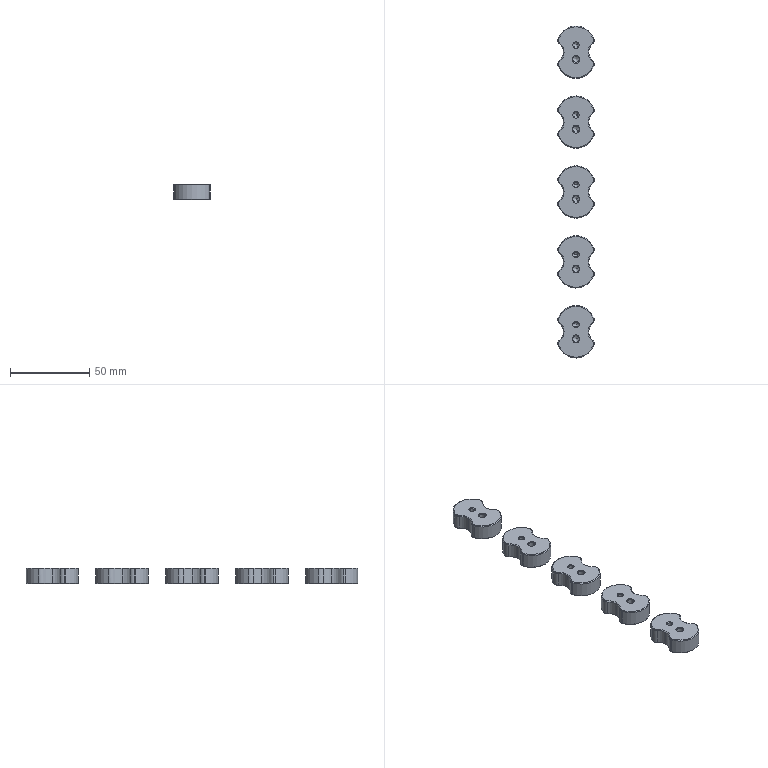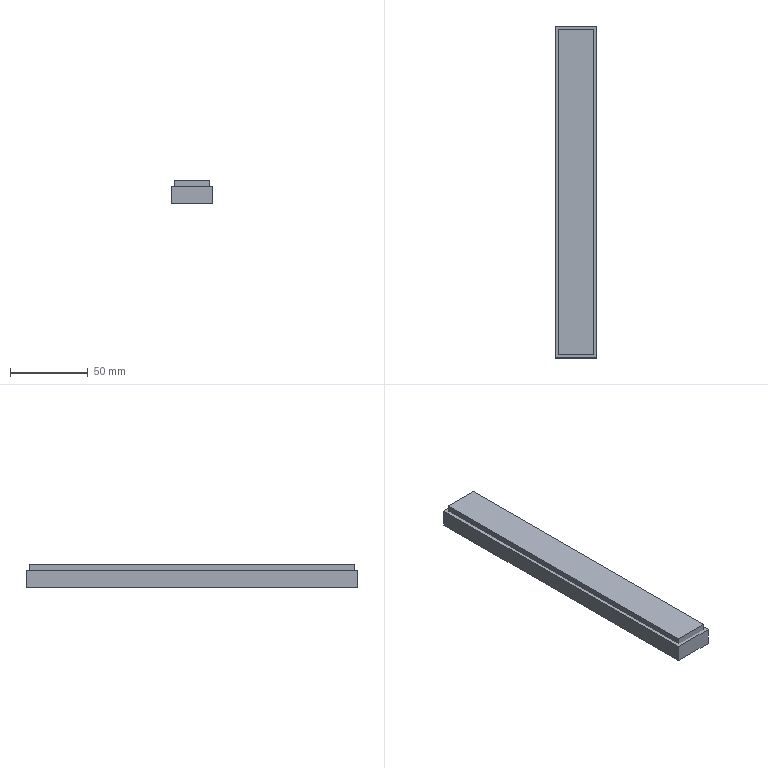CAM job | NX | 3-axis milling | part box 22.923 x 209 x 10 mm | stock box 26.923 x 213 x 15 mm
Tools:
number,name,description,diameter,corner_radius,flute_length,length,flutes
19,D80,Milling Tool-5 Parameters,80.0,0.0,50.0,75.0,2
15,D10,Milling Tool-5 Parameters,10.0,0.0,50.0,75.0,2
14,D10JING,Milling Tool-5 Parameters,10.0,0.0,50.0,75.0,2
1,D6A45,Milling Tool-5 Parameters,6.0,0.0,50.0,75.0,2
17,D2,Milling Tool-5 Parameters,2.0,0.0,50.0,75.0,2
Operations:
program,operation,operation_type,tool,method,geometry_group,spindle_rpm,surface_speed,feed_per_tooth,feed_cut,feed_plunge,cut_length_mm,path_length_mm,cut_time_min,machine_time_min
1,FLOOR_WALL,VolumeBased25DMillingOperation,D80,METHOD,A,6500.0,1633.0,0.1154,1500.0,100.0,305.0,359.0,0.2033,0.2087
1,ZLEVEL_PROFILE_COPY_1,ZLevelMilling,D10,METHOD,A,9500.0,298.0,0.1842,3500.0,1000.0,7354.077,8159.199,2.272,2.352
1,ZLEVEL_PROFILE_COPY_1_COPY,ZLevelMilling,D10JING,METHOD,A,9500.0,298.0,0.0632,1200.0,1000.0,668.759,1593.239,0.5594,0.6519
1,HOLE_MILLING,CylinderMilling,D2,METHOD,A,9500.0,44.0,0.0303,1150.0,100.0,3125.391,3975.391,2.718,2.803
1,PLANAR_MILL_COPY_COPY_COPY_COPY,PlanarMilling,D6A45,METHOD,A,9500.0,179.0,0.0658,1250.0,100.0,635.76,1849.529,0.5086,0.63
1,TOOLCOMP15,CylinderMilling,D2,METHOD,A,9500.0,44.0,0.0303,1150.0,100.0,405.424,1255.424,0.3525,0.4375
2,FLOOR_WALL_COPY,VolumeBased25DMillingOperation,D80,METHOD,B,6500.0,1633.0,0.1154,1500.0,100.0,3050.0,6236.003,2.033,2.352
2,PLANAR_MILL_COPY_COPY_COPY_COPY_COPY,PlanarMilling,D6A45,METHOD,B,9500.0,179.0,0.0658,1250.0,100.0,542.929,1055.031,0.4343,0.4856